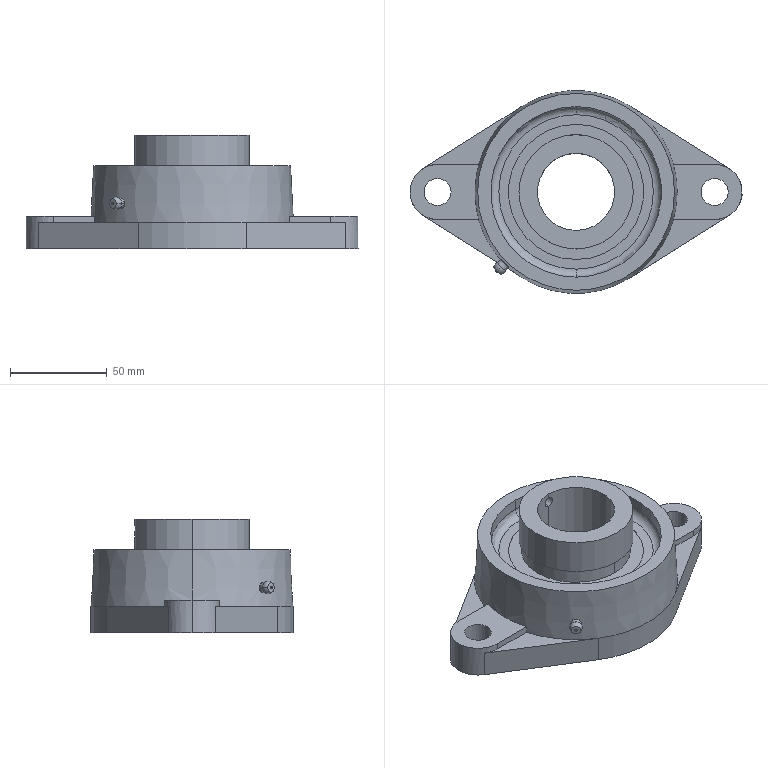Part | STEP file | 1 solid | 123 faces | box 172 x 105 x 58.9 mm | volume 260417 mm3 | cylinder 44 | sphere 36 | plane 35 | torus 6 | cone 2 | commonest cylinder face diameters 6 x6 28.5 x6 70 x6 14 x4 56.4 x4 88.333 x4